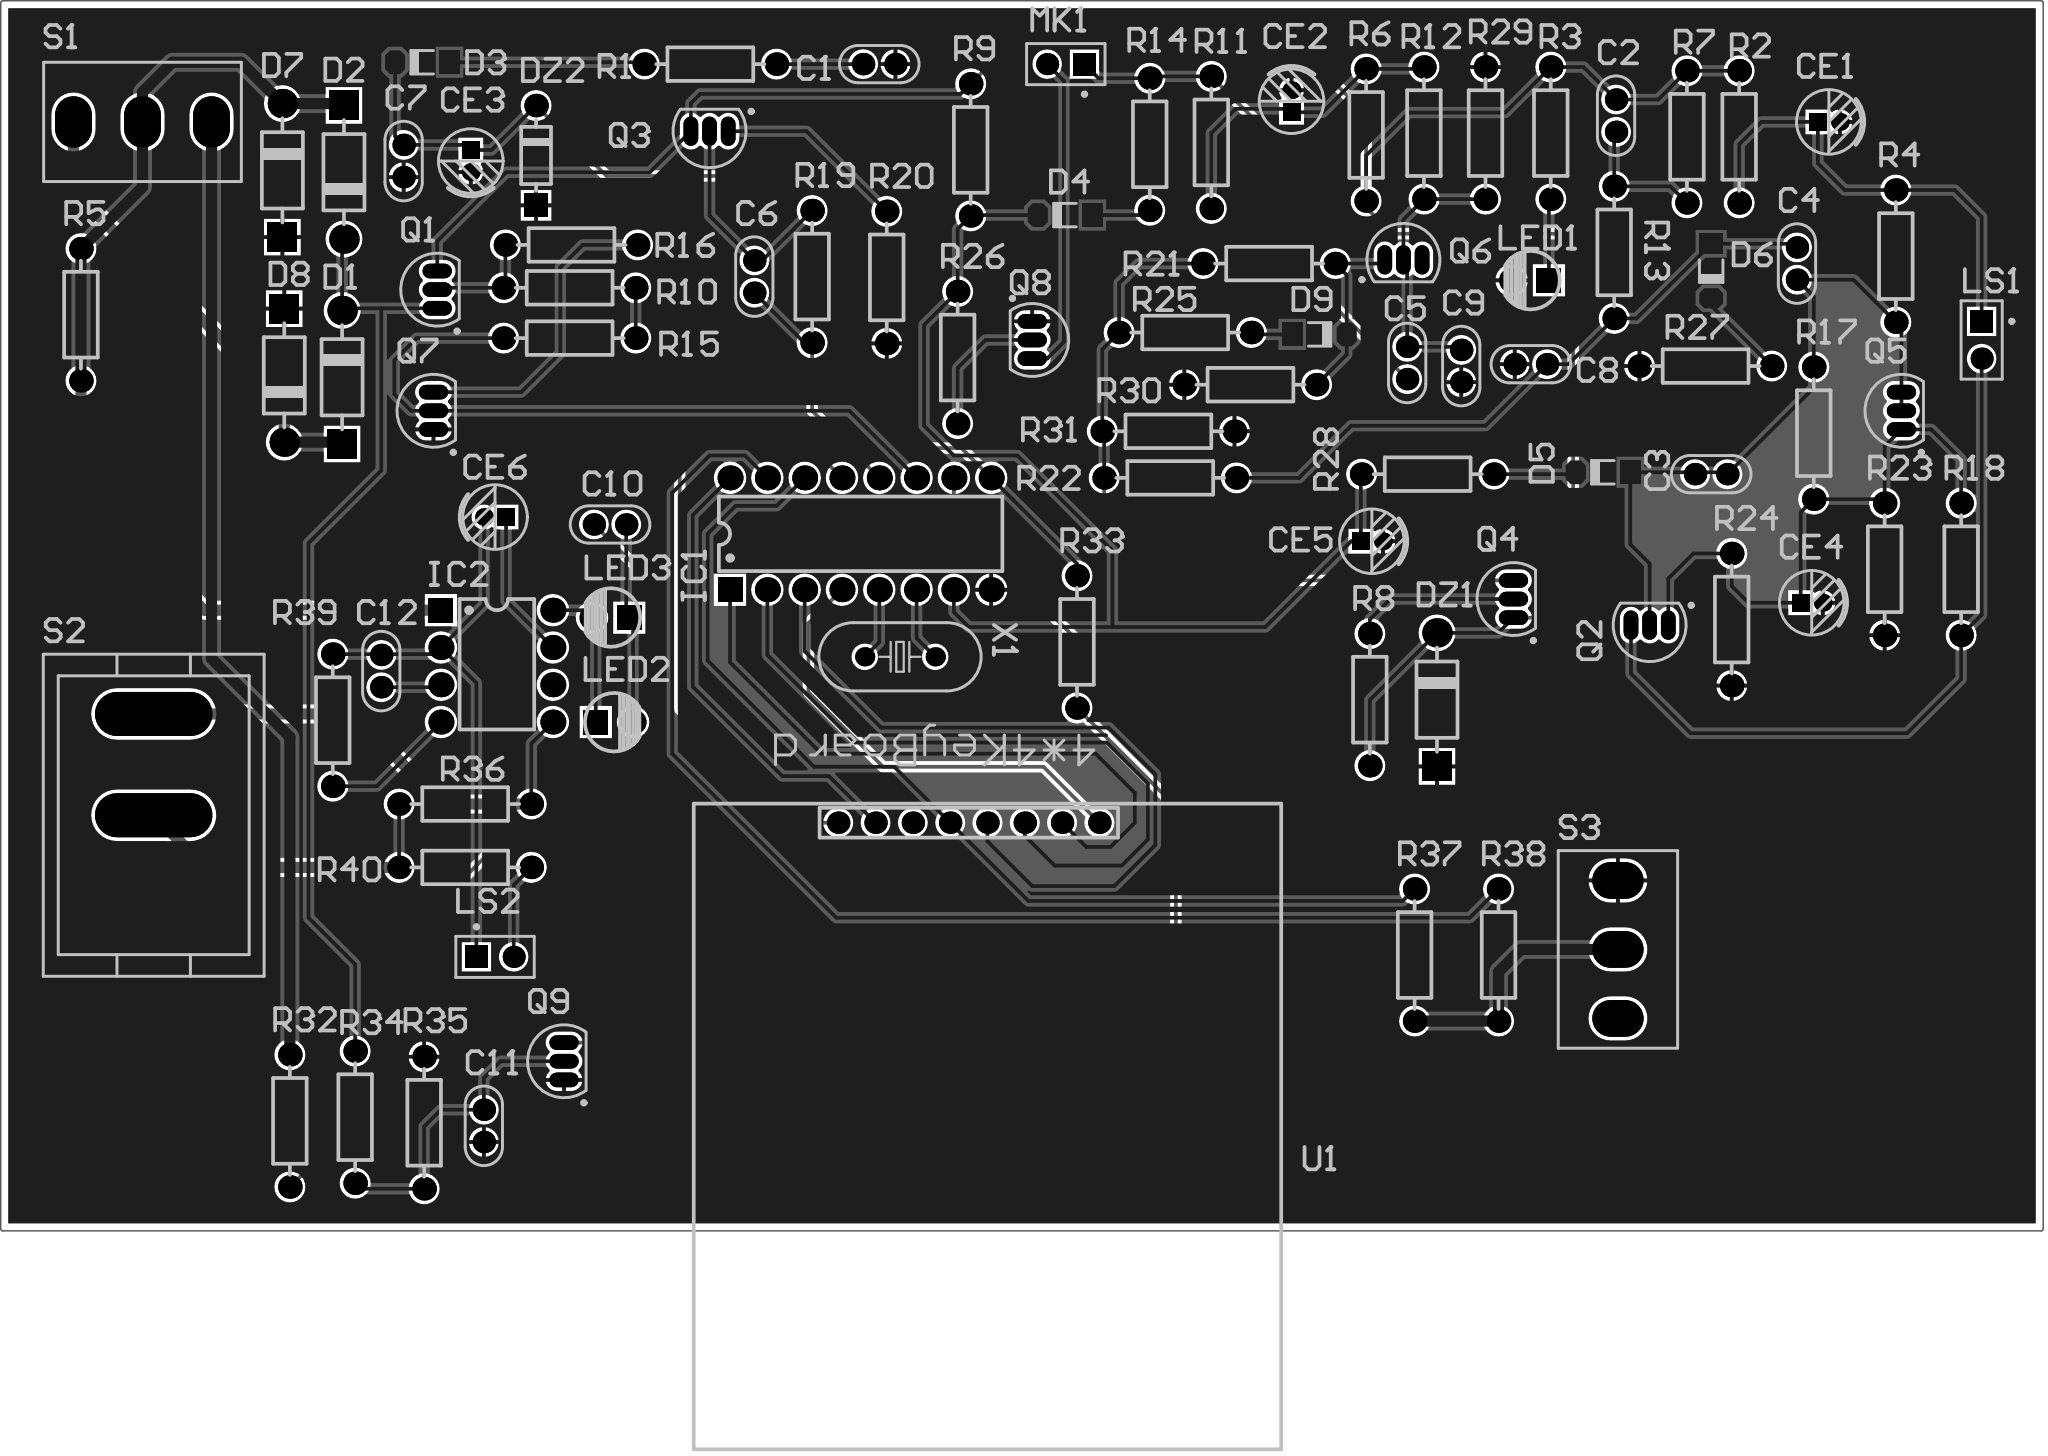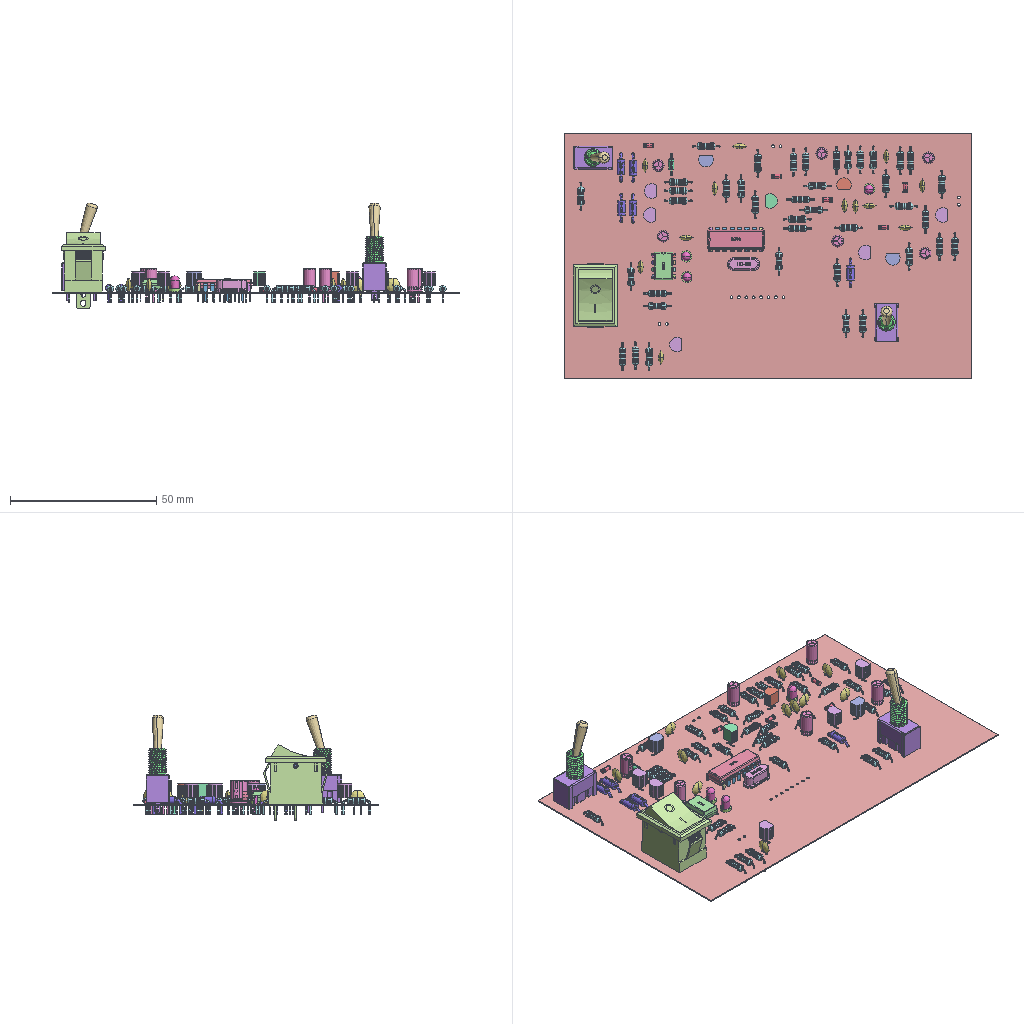Circuit board layout | Altium Designer | box 139.1 x 83.8 x 36.3 mm
Layer stack:
# Altium Designer layer stack of  (unit mm; dielectric type: 0 none, 1 core, 2 prepreg, 3 surface material)
index,name,kind,layer,copper_thickness_mm,dielectric_type,dielectric_thickness_mm,dielectric_material,dielectric_constant
0,Top Paste,other,,,,,,
1,Top Overlay,other,,,,,,
2,Top Solder,dielectric,,,3,0.0102,Solder Resist,3.5
3,Top Layer,copper,Top Layer,0.0356,,,,
4,Dielectric 1,dielectric,,,0,0.32,FR-4,4.8
5,Bottom Layer,copper,Bottom Layer,0.0356,,,,
6,Bottom Solder,dielectric,,,3,0.0102,Solder Resist,3.5
7,Bottom Overlay,other,,,,,,
8,Bottom Paste,other,,,,,,
# drill layer pairs: low layer,high layer
drill_pair,Top Layer,Bottom Layer
Part placement:
Designator,Comment,Layer,Footprint,Center-X(mm),Center-Y(mm),Rotation
X1,3.58MHZ,TopLayer,OSC_HC-49S,105.804,115.824,360
U1,4*4 matrix keypad,TopLayer,4*4_KEYBOARD,110.49,104.521,180
S3,MTS-10x,TopLayer,MTS-10x,154.686,95.885,90
S2,KCD1-101,TopLayer,KCD1-101,54.991,108.479,90
S1,MTS-10x,TopLayer,MTS-10x,54.229,152.273,360
R40,1K5,TopLayer,RS_1/4W,76.2,101.473,180
R39,33K,TopLayer,RS_1/4W,67.183,111.506,270
R38,820K,TopLayer,RS_1/4W,146.558,95.504,90
R37,820K,TopLayer,RS_1/4W,140.843,95.504,90
R36,7K5,TopLayer,RS_1/4W,76.2,105.791,360
R35,470k,TopLayer,RS_1/4W,73.406,84.074,270
R34,470k,TopLayer,RS_1/4W,68.707,84.455,90
R33,470k,TopLayer,RS_1/4W,117.856,116.84,90
R32,1K5,TopLayer,RS_1/4W,64.262,84.201,90
R31,18,TopLayer,RS_1/4W,124.079,131.191,180
R30,75K,TopLayer,RS_1/4W,129.667,134.366,180
R29,27K,TopLayer,RS_1/4W,145.669,151.511,90
R28,2K,TopLayer,RS_1/4W,141.732,128.27,180
R27,100,TopLayer,RS_1/4W,160.655,135.636,180
R26,100K,TopLayer,RS_1/4W,109.728,136.216,90
R25,100,TopLayer,RS_1/4W,125.222,137.922,180
R24,510,TopLayer,RS_1/4W,162.433,118.364,90
R23,150,TopLayer,RS_1/4W,172.847,121.793,90
R22,560,TopLayer,RS_1/4W,124.206,128.016,180
R21,470,TopLayer,RS_1/4W,130.937,142.621,180
R20,120,TopLayer,RS_1/4W,104.902,141.677,90
R19,5K1,TopLayer,RS_1/4W,99.822,141.732,90
R18,6k2,TopLayer,RS_1/4W,178.054,121.793,90
R17,20K,TopLayer,RS_1/4W,168.021,131.064,90
R16,5K1,TopLayer,RS_1/4W,83.439,143.891,180
R15,200K,TopLayer,RS_1/4W,83.312,137.541,180
R14,10K,TopLayer,RS_1/4W,122.809,150.749,270
R13,5K1,TopLayer,RS_1/4W,154.432,143.383,270
R12,130K,TopLayer,RS_1/4W,141.478,151.511,270
R11,2K,TopLayer,RS_1/4W,127,150.876,90
R10,100K,TopLayer,RS_1/4W,83.312,140.97,360
R9,33K,TopLayer,RS_1/4W,110.617,150.368,90
R8,10K,TopLayer,RS_1/4W,137.795,112.903,90
R7,9K1,TopLayer,RS_1/4W,159.385,151.257,270
R6,15K,TopLayer,RS_1/4W,137.541,151.384,90
R5,151V,TopLayer,RS_1/4W,50.038,139.137,90
R4,10K,TopLayer,RS_1/4W,173.609,143.129,90
R3,4K7,TopLayer,RS_1/4W,150.114,151.511,270
R2,1K2,TopLayer,RS_1/4W,162.941,151.257,270
R1,2K2,TopLayer,RS_1/4W,92.892,156.21,180
Q9,9014,TopLayer,TO-92A,82.931,88.265,0
Q8,5551,TopLayer,TO-92A,114.808,137.414,180
Q7,5551,TopLayer,TO-92A,74.041,132.588,360
Q6,9014,TopLayer,TO-92A,140.081,142.875,270
Q5,9014,TopLayer,TO-92A,173.99,132.588,0
Q4,A1013,TopLayer,TO-92A,147.574,119.761,360
Q3,5551,TopLayer,TO-92A,92.837,151.638,90
Q2,9014,TopLayer,TO-92A,156.845,117.983,90
Q1,A1013,TopLayer,TO-92A,74.295,140.843,360
MK1,Mic2,TopLayer,PIN2,117.094,156.21,180
LS2,Bell,TopLayer,PIN2,78.232,95.377,360
LS1,Speaker,TopLayer,PIN2,179.451,137.414,270
LED3,Red,TopLayer,LED_3MM-B,86.106,118.491,180
LED2,Red,TopLayer,LED_3MM-B,86.36,111.379,360
LED1,Red,TopLayer,LED_3MM-B,148.717,141.478,180
IC2,GL6840A,TopLayer,DIP8,78.359,115.189,0
IC1,HM91710A,TopLayer,DIP16,103.124,124.206,90
DZ2,1N4106,TopLayer,DO-35,81.026,149.987,90
DZ1,1N4742,TopLayer,DO-41,142.367,112.903,90
D9,1N4148,TopLayer,MINI_MELF_(LL34),134.366,137.795,360
D8,1N4007,TopLayer,DO-41,63.881,135.001,270
D7,1N4007,TopLayer,DO-41,63.754,148.971,90
D6,1N4148,TopLayer,MINI_MELF_(LL34),161.036,142.113,270
D5,1N4148,TopLayer,MINI_MELF_(LL34),153.67,128.397,180
D4,1N4148,TopLayer,MINI_MELF_(LL34),117.044,145.923,180
D3,1N4148,TopLayer,MINI_MELF_(LL34),73.279,156.337,180
D2,1N4007,TopLayer,DO-41,67.945,148.844,270
D1,1N4007,TopLayer,DO-41,67.818,134.874,90
CE6,10uF/16V,TopLayer,CAP_1.5*4*8,78.232,125.349,180
CE5,4.7UF,TopLayer,CAP_1.5*4*8,137.934,123.698,0
CE4,47UF,TopLayer,CAP_1.5*4*8,167.882,119.507,0
CE3,100UF,TopLayer,CAP_1.5*4*8,76.581,149.606,270
CE2,4.7UF,TopLayer,CAP_1.5*4*8,132.461,153.682,90
CE1,100UF,TopLayer,CAP_1.5*4*8,169.049,152.273,0
C12,100NF,TopLayer,CC_2.2*5,70.485,114.851,270
C11,100NF,TopLayer,CC_2.2*5,77.47,83.863,90
C10,1UF,TopLayer,CC_2.2*5,86.063,124.841,360
C9,33NF,TopLayer,CC_2.2*5,144.018,135.636,90
C8,22NF,TopLayer,CC_2.2*5,148.76,135.763,360
C7,100NF,TopLayer,CC_2.2*5,72.009,149.606,90
C6,22NF,TopLayer,CC_2.2*5,95.885,141.732,90
C5,10NF,TopLayer,CC_2.2*5,140.335,135.847,270
C4,100NF,TopLayer,CC_2.2*5,166.878,142.621,90
C3,100NF,TopLayer,CC_2.2*5,161.036,128.27,180
C2,10NF,TopLayer,CC_2.2*5,154.559,152.697,90
C1,22NF,TopLayer,CC_2.2*5,104.394,156.21,180
Pad and via stacks:
# Altium Designer via and pad stacks of  (unit mm). Each distinct definition once, with the count of objects using it.
# via: kind,start_layer,end_layer,hole_mm,diameter_mm,mode(0 simple;1 top-mid-bottom;2 full stack),diameter_per_layer,count,example_net
# pad: kind,layer,hole_mm,hole_type(0 round;1 square;2 slot),plating,top_size,top_shape(1 round;2 rect;3 octagon;9 rounded rect),mid_size,bottom_size,mode,footprint,size_per_layer,count,example
pad,Multi-Layer,0.6,0,plated,1.6x1.6,1,1.6x1.6,1.6x1.6,0,RS 1/4W,,80,R1.2
pad,Multi-Layer,0.9,0,plated,1.5x1.5,2,1.5x1.5,1.5x1.5,0,PIN2,,3,LS1.1
pad,Multi-Layer,0.9,0,plated,1.5x1.5,1,1.5x1.5,1.5x1.5,0,PIN2,,3,LS1.2
pad,Multi-Layer,0.9,0,plated,2x1,1,2x1,2x1,0,TO-92A,,27,Q1.3
pad,Multi-Layer,1,2,unplated,3.5x2.5,1,3.5x2.5,3.5x2.5,0,MTS-10x,,6,S1.1
pad,Multi-Layer,0.6,0,plated,1.2x1.2,1,1.2x1.2,1.2x1.2,0,CAP 1.5*4*8,,6,CE1.2
pad,Multi-Layer,0.6,0,plated,1.2x1.2,2,1.2x1.2,1.2x1.2,0,CAP 1.5*4*8,,6,CE1.1
pad,Multi-Layer,1,0,plated,2x2,1,2x2,2x2,0,DO-41,,5,DZ1.2
pad,Multi-Layer,1,0,plated,2x2,2,2x2,2x2,0,DO-41,,5,DZ1.1
pad,Multi-Layer,0.5,0,plated,1.524x1.524,1,1.524x1.524,1.524x1.524,0,CC 2.2*5,,24,C1.2
pad,Multi-Layer,0.9,0,plated,1.7x1.7,2,1.7x1.7,1.7x1.7,0,LED 3MM-B,,3,LED1.1
pad,Multi-Layer,0.9,0,plated,1.7x1.7,1,1.7x1.7,1.7x1.7,0,LED 3MM-B,,3,LED1.2
pad,Multi-Layer,0.8,0,plated,1.6x1.6,1,1.6x1.6,1.6x1.6,0,DO-35,,1,DZ2.2
pad,Multi-Layer,0.8,0,plated,1.6x1.6,2,1.6x1.6,1.6x1.6,0,DO-35,,1,DZ2.1
pad,Multi-Layer,0.8,0,plated,1.7x1.7,1,1.7x1.7,1.7x1.7,0,DIP16,,15,IC1.16
pad,Multi-Layer,0.8,0,plated,1.7x1.7,2,1.7x1.7,1.7x1.7,0,DIP16,,1,IC1.1
pad,Multi-Layer,0.9144,0,plated,1.524x1.524,1,1.524x1.524,1.524x1.524,0,4*4 KEYBOARD,,8,U1.2
pad,Multi-Layer,0.8,0,plated,1.7x1.7,1,1.7x1.7,1.7x1.7,0,DIP8,,7,IC2.8
pad,Multi-Layer,0.8,0,plated,1.7x1.7,2,1.7x1.7,1.7x1.7,0,DIP8,,1,IC2.1
pad,Multi-Layer,0.6,0,plated,1.3x1.3,1,1.3x1.3,1.3x1.3,0,OSC HC-49S,,2,X1.2
pad,Multi-Layer,0.8,2,plated,3x8,1,3x8,3x8,0,KCD1-101,,2,S2.2
pad,Top Layer,0,0,plated,1.62x1.37,3,1.62x1.37,1.62x1.37,0,MINI_MELF (LL34),,5,D3.2
pad,Top Layer,0,0,plated,1.62x1.37,2,1.62x1.37,1.62x1.37,0,MINI_MELF (LL34),,5,D3.1
Copper pours:
name,layer,net,type(0 solid;1 hatched;2 none)
D,Top Layer,GND,0
D,Bottom Layer,GND,0
Design rules, without the lines most boards share:
# Altium Designer design rules of  (exported by Altium Designer, unit mm)
# columns: name | kind | enabled | priority | scope1 | scope2 | descriptor | typed fields (field=value)
SilkToSilkClearance | 55 | enabled | 1 | All | All | Silk to Silk (Clearance=0mil) (All),(All) |
SilkToSolderMaskClearance | 54 | enabled | 1 | IsPad | All | Silk To Solder Mask (Clearance=0mil) (IsPad),(All) |
MinimumSolderMaskSliver | 53 | enabled | 1 | All | All | Minimum Solder Mask Sliver (Gap=0mil) (All),(All) |
HoleToHoleClearance | 52 | enabled | 1 | All | All | Hole To Hole Clearance (Gap=10mil) (All),(All) | gap=0.254
DiffPairsRouting | 51 | enabled | 1 | All | All | Differential Pairs Uncoupled Length using the Gap Constraints (Min=10mil) (Max=10mil) (Prefered=10mil)  and Width Constraints (Min=15mil) (Max=15mil) (Prefered=15mil) (All) |
HoleSize | 42 | enabled | 1 | All | All | Hole Size Constraint (Min=1mil) (Max=1000mil) (All) |
Height | 50 | enabled | 1 | All | All | Height Constraint (Min=0mil) (Max=99999mil) (Prefered=500mil) (All) | min_height=0 max_height=2539.975
SolderMaskExpansion | 13 | enabled | 1 | All | All | Solder Mask Expansion (Expansion =4mil) (All) | expansion=0.1016
PasteMaskExpansion | 14 | enabled | 1 | All | All | Paste Mask Expansion (Expansion =0mil) (All) | expansion=0
RoutingVias | 11 | enabled | 1 | All | All | Routing Via (MinHoleWidth=28mil) (MaxHoleWidth=28mil) (PreferredHoleWidth=28mil) (MinWidth=50mil) (MaxWidth=50mil) (PreferedWidth=50mil) (All) | via_min_hole=0.7112 via_max_hole=0.7112 via_preferred_diameter=1.27 via_preferred_hole=0.7112
Width | 2 | enabled | 1 | All | All | Width Constraint (Min=10mil) (Max=30mil) (Preferred=10mil) (All) |
PolygonConnect | 20 | enabled | 1 | All | All | Polygon Connect Rule(Relief Connect )(Conductor Width=10mil) (Relief Angle=90 Angle) (Entries=4) (Air Gap Width=10mil) (All),(All) | connect_style(0=relief,1=direct,2=none)=0 relief_conductor_width=0.254 relief_entries=4
PlaneConnect | 6 | enabled | 1 | All | All | Power Plane Connect Rule(Relief Connect )(Expansion=20mil) (Conductor Width=10mil) (Air Gap=10mil) (Entries=4) (All) | relief_conductor_width=0.254 relief_entries=4 relief_expansion=0.508
Clearance | 0 | enabled | 1 | All | All | Clearance Constraint (Gap=10mil) (All),(All) | gap=0.254
Classes set for this board:
# Altium Designer classes of  (member kind: 0 net, 1 component, 2 from-to, 3 pad, 4 layer, 5 differential pair, 6 design channel, 7 polygon, 8 structure, 9 xSignal)
# columns: class name | member kind | superclass | members
Sheet1 | 1 | no | C1; C2; C3; C4; C5; C6; C7; C8; C9; C10; C11; C12; CE1; CE2; CE3; CE4; CE5; CE6; D1; D2; D3; D4; D5; D6; D7; D8; D9; DZ1; DZ2; IC1; IC2; LED1; LED2; LED3; LS1; LS2; MK1; Q1; Q2; Q3; Q4; Q5; Q6; Q7; Q8; Q9; R1; R2; R3; R4; R5; R6; R7; R8; R9; R10; R11; R12; R13; R14; R15; R16; R17; R18; R19; R20; R21; R22; R23; R24; R25; R26; R27; R28; R29; R30; R31; R32; R33; R34; R35; R36; R37; R38; R39; R40; S1; S2; S3; U1; X1;